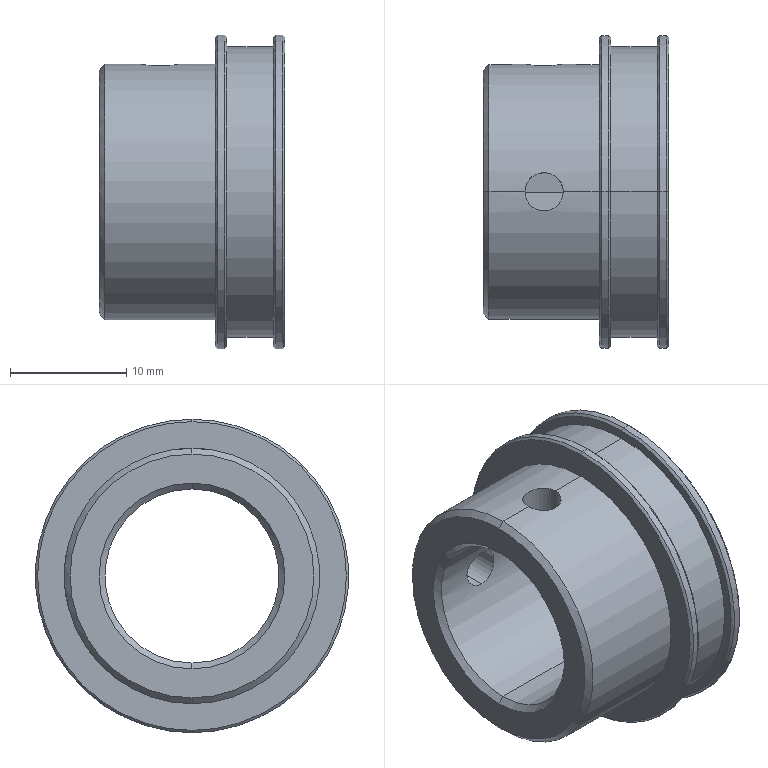Part | SolidWorks | features ICE 3, Chamfer 2, HoleWzd 2, Extrusion 1 | 1 solid | 33 faces | box 16 x 27 x 27 mm | volume 3995 mm3 | cylinder 14 | cone 14 | plane 5 | commonest cylinder face diameters 3.3 x4 27 x4 15 x2 22 x2 25 x2
STEP:
#1=CARTESIAN_POINT('',(-4.1,0.,11.));
#2=VERTEX_POINT('',#1);
#3=CARTESIAN_POINT('',(-7.4,0.,11.));
#4=VERTEX_POINT('',#3);
#5=CARTESIAN_POINT('',(-4.1,0.,11.));
#6=CARTESIAN_POINT('',(-4.1,-0.2155,11.));
#7=CARTESIAN_POINT('',(-4.143,-0.4328,10.993));
#8=CARTESIAN_POINT('',(-4.308,-0.83,10.97));
#9=CARTESIAN_POINT('',(-4.431,-1.014,10.954));
#10=CARTESIAN_POINT('',(-4.659,-1.242,10.93));
#11=CARTESIAN_POINT('',(-4.743,-1.312,10.922));
#12=CARTESIAN_POINT('',(-4.922,-1.431,10.907));
#13=CARTESIAN_POINT('',(-5.017,-1.482,10.9));
#14=CARTESIAN_POINT('',(-5.217,-1.565,10.888));
#15=CARTESIAN_POINT('',(-5.321,-1.597,10.883));
#16=CARTESIAN_POINT('',(-5.532,-1.639,10.877));
#17=CARTESIAN_POINT('',(-5.64,-1.65,10.876));
#18=CARTESIAN_POINT('',(-5.858,-1.65,10.876));
#19=CARTESIAN_POINT('',(-5.965,-1.639,10.877));
#20=CARTESIAN_POINT('',(-6.176,-1.598,10.883));
#21=CARTESIAN_POINT('',(-6.281,-1.566,10.888));
#22=CARTESIAN_POINT('',(-6.481,-1.483,10.9));
#23=CARTESIAN_POINT('',(-6.576,-1.433,10.906));
#24=CARTESIAN_POINT('',(-6.755,-1.313,10.922));
#25=CARTESIAN_POINT('',(-6.84,-1.243,10.93));
#26=CARTESIAN_POINT('',(-7.068,-1.016,10.954));
#27=CARTESIAN_POINT('',(-7.191,-0.832,10.97));
#28=CARTESIAN_POINT('',(-7.356,-0.4352,10.993));
#29=CARTESIAN_POINT('',(-7.4,-0.2183,11.));
#30=CARTESIAN_POINT('',(-7.4,0.,11.));
#31=B_SPLINE_CURVE_WITH_KNOTS('',3,(#5,#6,#7,#8,#9,#10,#11,#12,#13,#14,#15,#16,#17,#18,#19,#20,#21,#22,#23,#24,#25,#26,#27,#28,#29,#30),.UNSPECIFIED.,.F.,.F.,(4,2,2,2,2,2,2,2,2,2,2,2,4),(0.005166,0.005812,0.006457,0.00678,0.007103,0.007425,0.007748,0.008071,0.008394,0.008717,0.009039,0.009685,0.01033),.UNSPECIFIED.);
#32=EDGE_CURVE('',#2,#4,#31,.T.);
#33=ORIENTED_EDGE('',*,*,#32,.F.);
#34=CARTESIAN_POINT('',(-4.1,0.,7.5));
#35=VERTEX_POINT('',#34);
#36=CARTESIAN_POINT('',(-4.1,0.,0.));
#37=DIRECTION('',(0.,0.,-1.));
#38=VECTOR('',#37,1000.);
#39=LINE('',#36,#38);
#40=EDGE_CURVE('',#2,#35,#39,.T.);
#41=ORIENTED_EDGE('',*,*,#40,.T.);
#42=CARTESIAN_POINT('',(-7.4,0.,7.5));
#43=VERTEX_POINT('',#42);
#44=CARTESIAN_POINT('',(-4.1,0.,7.5));
#45=CARTESIAN_POINT('',(-4.1,-0.1094,7.5));
#46=CARTESIAN_POINT('',(-4.111,-0.2169,7.498));
#47=CARTESIAN_POINT('',(-4.153,-0.4282,7.489));
#48=CARTESIAN_POINT('',(-4.185,-0.5332,7.482));
#49=CARTESIAN_POINT('',(-4.268,-0.7329,7.465));
#50=CARTESIAN_POINT('',(-4.318,-0.8275,7.455));
#51=CARTESIAN_POINT('',(-4.438,-1.007,7.433));
#52=CARTESIAN_POINT('',(-4.508,-1.091,7.421));
#53=CARTESIAN_POINT('',(-4.735,-1.319,7.385));
#54=CARTESIAN_POINT('',(-4.919,-1.442,7.361));
#55=CARTESIAN_POINT('',(-5.316,-1.606,7.326));
#56=CARTESIAN_POINT('',(-5.533,-1.65,7.316));
#57=CARTESIAN_POINT('',(-5.857,-1.65,7.316));
#58=CARTESIAN_POINT('',(-5.967,-1.639,7.319));
#59=CARTESIAN_POINT('',(-6.179,-1.597,7.328));
#60=CARTESIAN_POINT('',(-6.282,-1.566,7.335));
#61=CARTESIAN_POINT('',(-6.582,-1.441,7.361));
#62=CARTESIAN_POINT('',(-6.764,-1.32,7.385));
#63=CARTESIAN_POINT('',(-6.993,-1.09,7.421));
#64=CARTESIAN_POINT('',(-7.061,-1.007,7.433));
#65=CARTESIAN_POINT('',(-7.181,-0.8286,7.455));
#66=CARTESIAN_POINT('',(-7.233,-0.7319,7.465));
#67=CARTESIAN_POINT('',(-7.315,-0.5325,7.482));
#68=CARTESIAN_POINT('',(-7.347,-0.4297,7.488));
#69=CARTESIAN_POINT('',(-7.389,-0.2174,7.498));
#70=CARTESIAN_POINT('',(-7.4,-0.1079,7.5));
#71=CARTESIAN_POINT('',(-7.4,0.,7.5));
#72=B_SPLINE_CURVE_WITH_KNOTS('',3,(#44,#45,#46,#47,#48,#49,#50,#51,#52,#53,#54,#55,#56,#57,#58,#59,#60,#61,#62,#63,#64,#65,#66,#67,#68,#69,#70,#71),.UNSPECIFIED.,.F.,.F.,(4,2,2,2,2,2,2,2,2,2,2,2,2,4),(0.,0.0003234,0.0006468,0.0009702,0.001294,0.00194,0.002587,0.002911,0.003234,0.003881,0.004204,0.004528,0.004851,0.005175),.UNSPECIFIED.);
#73=EDGE_CURVE('',#35,#43,#72,.T.);
#74=ORIENTED_EDGE('',*,*,#73,.T.);
#75=CARTESIAN_POINT('',(-7.4,0.,0.));
#76=DIRECTION('',(0.,0.,-1.));
#77=VECTOR('',#76,1000.);
#78=LINE('',#75,#77);
#79=EDGE_CURVE('',#4,#43,#78,.T.);
#80=ORIENTED_EDGE('',*,*,#79,.F.);
#81=EDGE_LOOP('',(#33,#41,#74,#80));
#82=FACE_OUTER_BOUND('',#81,.T.);
#83=CARTESIAN_POINT('',(-5.75,0.,0.));
#84=DIRECTION('',(0.,0.,-1.));
#85=DIRECTION('',(-1.,0.,0.));
#86=AXIS2_PLACEMENT_3D('',#83,#84,#85);
#87=CYLINDRICAL_SURFACE('',#86,1.65);
#88=ADVANCED_FACE('',(#82),#87,.F.);
#89=CARTESIAN_POINT('',(-5.75,10.876,1.65));
#90=VERTEX_POINT('',#89);
#91=CARTESIAN_POINT('',(-5.75,10.876,-1.65));
#92=VERTEX_POINT('',#91);
#93=CARTESIAN_POINT('',(-5.75,10.876,1.65));
#94=CARTESIAN_POINT('',(-5.965,10.876,1.65));
#95=CARTESIAN_POINT('',(-6.183,10.882,1.607));
#96=CARTESIAN_POINT('',(-6.58,10.905,1.442));
#97=CARTESIAN_POINT('',(-6.764,10.922,1.319));
#98=CARTESIAN_POINT('',(-6.992,10.946,1.092));
#99=CARTESIAN_POINT('',(-7.062,10.954,1.007));
#100=CARTESIAN_POINT('',(-7.181,10.969,0.8278));
#101=CARTESIAN_POINT('',(-7.232,10.976,0.7332));
#102=CARTESIAN_POINT('',(-7.315,10.988,0.5333));
#103=CARTESIAN_POINT('',(-7.347,10.992,0.4286));
#104=CARTESIAN_POINT('',(-7.389,10.998,0.2177));
#105=CARTESIAN_POINT('',(-7.4,11.,0.1101));
#106=CARTESIAN_POINT('',(-7.4,11.,-0.108));
#107=CARTESIAN_POINT('',(-7.389,10.998,-0.2152));
#108=CARTESIAN_POINT('',(-7.348,10.992,-0.4264));
#109=CARTESIAN_POINT('',(-7.316,10.988,-0.5314));
#110=CARTESIAN_POINT('',(-7.233,10.976,-0.731));
#111=CARTESIAN_POINT('',(-7.183,10.969,-0.8258));
#112=CARTESIAN_POINT('',(-7.063,10.954,-1.005));
#113=CARTESIAN_POINT('',(-6.993,10.946,-1.09));
#114=CARTESIAN_POINT('',(-6.766,10.922,-1.318));
#115=CARTESIAN_POINT('',(-6.582,10.906,-1.441));
#116=CARTESIAN_POINT('',(-6.185,10.882,-1.606));
#117=CARTESIAN_POINT('',(-5.968,10.876,-1.65));
#118=CARTESIAN_POINT('',(-5.75,10.876,-1.65));
#119=B_SPLINE_CURVE_WITH_KNOTS('',3,(#93,#94,#95,#96,#97,#98,#99,#100,#101,#102,#103,#104,#105,#106,#107,#108,#109,#110,#111,#112,#113,#114,#115,#116,#117,#118),.UNSPECIFIED.,.F.,.F.,(4,2,2,2,2,2,2,2,2,2,2,2,4),(0.005166,0.005812,0.006457,0.00678,0.007103,0.007425,0.007748,0.008071,0.008394,0.008717,0.009039,0.009685,0.01033),.UNSPECIFIED.);
#120=EDGE_CURVE('',#90,#92,#119,.T.);
#121=ORIENTED_EDGE('',*,*,#120,.F.);
#122=CARTESIAN_POINT('',(-5.75,7.316,1.65));
#123=VERTEX_POINT('',#122);
#124=CARTESIAN_POINT('',(-5.75,0.,1.65));
#125=DIRECTION('',(0.,-1.,0.));
#126=VECTOR('',#125,1000.);
#127=LINE('',#124,#126);
#128=EDGE_CURVE('',#90,#123,#127,.T.);
#129=ORIENTED_EDGE('',*,*,#128,.T.);
#130=CARTESIAN_POINT('',(-5.75,7.316,-1.65));
#131=VERTEX_POINT('',#130);
#132=CARTESIAN_POINT('',(-5.75,7.316,1.65));
#133=CARTESIAN_POINT('',(-5.966,7.316,1.65));
#134=CARTESIAN_POINT('',(-6.183,7.326,1.607));
#135=CARTESIAN_POINT('',(-6.481,7.352,1.483));
#136=CARTESIAN_POINT('',(-6.578,7.362,1.431));
#137=CARTESIAN_POINT('',(-6.757,7.385,1.311));
#138=CARTESIAN_POINT('',(-6.84,7.397,1.243));
#139=CARTESIAN_POINT('',(-6.992,7.421,1.091));
#140=CARTESIAN_POINT('',(-7.062,7.433,1.007));
#141=CARTESIAN_POINT('',(-7.181,7.455,0.8283));
#142=CARTESIAN_POINT('',(-7.232,7.465,0.7337));
#143=CARTESIAN_POINT('',(-7.357,7.49,0.4332));
#144=CARTESIAN_POINT('',(-7.4,7.5,0.2185));
#145=CARTESIAN_POINT('',(-7.4,7.5,-0.1082));
#146=CARTESIAN_POINT('',(-7.389,7.498,-0.2155));
#147=CARTESIAN_POINT('',(-7.347,7.489,-0.4271));
#148=CARTESIAN_POINT('',(-7.315,7.482,-0.5324));
#149=CARTESIAN_POINT('',(-7.192,7.456,-0.8312));
#150=CARTESIAN_POINT('',(-7.069,7.433,-1.014));
#151=CARTESIAN_POINT('',(-6.766,7.385,-1.318));
#152=CARTESIAN_POINT('',(-6.583,7.361,-1.441));
#153=CARTESIAN_POINT('',(-6.285,7.335,-1.565));
#154=CARTESIAN_POINT('',(-6.18,7.328,-1.597));
#155=CARTESIAN_POINT('',(-5.967,7.319,-1.639));
#156=CARTESIAN_POINT('',(-5.859,7.316,-1.65));
#157=CARTESIAN_POINT('',(-5.75,7.316,-1.65));
#158=B_SPLINE_CURVE_WITH_KNOTS('',3,(#132,#133,#134,#135,#136,#137,#138,#139,#140,#141,#142,#143,#144,#145,#146,#147,#148,#149,#150,#151,#152,#153,#154,#155,#156,#157),.UNSPECIFIED.,.F.,.F.,(4,2,2,2,2,2,2,2,2,2,2,2,4),(0.005174,0.005821,0.006144,0.006468,0.006791,0.007114,0.007761,0.008084,0.008408,0.009054,0.009701,0.01002,0.01035),.UNSPECIFIED.);
#159=EDGE_CURVE('',#123,#131,#158,.T.);
#160=ORIENTED_EDGE('',*,*,#159,.T.);
#161=CARTESIAN_POINT('',(-5.75,0.,-1.65));
#162=DIRECTION('',(0.,-1.,0.));
#163=VECTOR('',#162,1000.);
#164=LINE('',#161,#163);
#165=EDGE_CURVE('',#92,#131,#164,.T.);
#166=ORIENTED_EDGE('',*,*,#165,.F.);
#167=EDGE_LOOP('',(#121,#129,#160,#166));
#168=FACE_OUTER_BOUND('',#167,.T.);
#169=CARTESIAN_POINT('',(-5.75,0.,0.));
#170=DIRECTION('',(0.,-1.,0.));
#171=DIRECTION('',(0.,0.,-1.));
#172=AXIS2_PLACEMENT_3D('',#169,#170,#171);
#173=CYLINDRICAL_SURFACE('',#172,1.65);
#174=ADVANCED_FACE('',(#168),#173,.F.);
#175=CARTESIAN_POINT('',(4.,0.,13.3));
#176=VERTEX_POINT('',#175);
#177=CARTESIAN_POINT('',(4.,0.,-13.3));
#178=VERTEX_POINT('',#177);
#179=CARTESIAN_POINT('',(4.,0.,0.));
#180=DIRECTION('',(-1.,0.,0.));
#181=DIRECTION('',(0.,0.,-1.));
#182=AXIS2_PLACEMENT_3D('',#179,#180,#181);
#183=CIRCLE('',#182,13.3);
#184=EDGE_CURVE('',#176,#178,#183,.T.);
#185=ORIENTED_EDGE('',*,*,#184,.F.);
#186=CARTESIAN_POINT('',(4.2,0.,13.5));
#187=VERTEX_POINT('',#186);
#188=CARTESIAN_POINT('',(4.2,0.,13.5));
#189=DIRECTION('',(0.7071,0.,0.7071));
#190=VECTOR('',#189,1000.);
#191=LINE('',#188,#190);
#192=EDGE_CURVE('',#176,#187,#191,.T.);
#193=ORIENTED_EDGE('',*,*,#192,.T.);
#194=CARTESIAN_POINT('',(4.2,0.,-13.5));
#195=VERTEX_POINT('',#194);
#196=CARTESIAN_POINT('',(4.2,0.,0.));
#197=DIRECTION('',(1.,0.,0.));
#198=DIRECTION('',(0.,0.,-1.));
#199=AXIS2_PLACEMENT_3D('',#196,#197,#198);
#200=CIRCLE('',#199,13.5);
#201=EDGE_CURVE('',#195,#187,#200,.T.);
#202=ORIENTED_EDGE('',*,*,#201,.F.);
#203=CARTESIAN_POINT('',(4.2,0.,-13.5));
#204=DIRECTION('',(0.7071,0.,-0.7071));
#205=VECTOR('',#204,1000.);
#206=LINE('',#203,#205);
#207=EDGE_CURVE('',#178,#195,#206,.T.);
#208=ORIENTED_EDGE('',*,*,#207,.F.);
#209=EDGE_LOOP('',(#185,#193,#202,#208));
#210=FACE_OUTER_BOUND('',#209,.T.);
#211=CARTESIAN_POINT('',(4.2,0.,0.));
#212=DIRECTION('',(1.,0.,0.));
#213=DIRECTION('',(0.,0.,-1.));
#214=AXIS2_PLACEMENT_3D('',#211,#212,#213);
#215=CONICAL_SURFACE('',#214,13.5,0.7854);
#216=ADVANCED_FACE('',(#210),#215,.T.);
#217=CARTESIAN_POINT('',(5.,0.,-13.3));
#218=VERTEX_POINT('',#217);
#219=CARTESIAN_POINT('',(5.,0.,13.3));
#220=VERTEX_POINT('',#219);
#221=CARTESIAN_POINT('',(5.,0.,0.));
#222=DIRECTION('',(1.,0.,0.));
#223=DIRECTION('',(0.,0.,-1.));
#224=AXIS2_PLACEMENT_3D('',#221,#222,#223);
#225=CIRCLE('',#224,13.3);
#226=EDGE_CURVE('',#218,#220,#225,.T.);
#227=ORIENTED_EDGE('',*,*,#226,.F.);
#228=CARTESIAN_POINT('',(4.8,0.,-13.5));
#229=VERTEX_POINT('',#228);
#230=CARTESIAN_POINT('',(5.,0.,-13.3));
#231=DIRECTION('',(-0.7071,0.,-0.7071));
#232=VECTOR('',#231,1000.);
#233=LINE('',#230,#232);
#234=EDGE_CURVE('',#218,#229,#233,.T.);
#235=ORIENTED_EDGE('',*,*,#234,.T.);
#236=CARTESIAN_POINT('',(4.8,0.,13.5));
#237=VERTEX_POINT('',#236);
#238=CARTESIAN_POINT('',(4.8,0.,0.));
#239=DIRECTION('',(-1.,0.,0.));
#240=DIRECTION('',(0.,0.,-1.));
#241=AXIS2_PLACEMENT_3D('',#238,#239,#240);
#242=CIRCLE('',#241,13.5);
#243=EDGE_CURVE('',#237,#229,#242,.T.);
#244=ORIENTED_EDGE('',*,*,#243,.F.);
#245=CARTESIAN_POINT('',(5.,0.,13.3));
#246=DIRECTION('',(-0.7071,0.,0.7071));
#247=VECTOR('',#246,1000.);
#248=LINE('',#245,#247);
#249=EDGE_CURVE('',#220,#237,#248,.T.);
#250=ORIENTED_EDGE('',*,*,#249,.F.);
#251=EDGE_LOOP('',(#227,#235,#244,#250));
#252=FACE_OUTER_BOUND('',#251,.T.);
#253=CARTESIAN_POINT('',(5.,0.,0.));
#254=DIRECTION('',(-1.,0.,0.));
#255=DIRECTION('',(0.,0.,1.));
#256=AXIS2_PLACEMENT_3D('',#253,#254,#255);
#257=CONICAL_SURFACE('',#256,13.3,0.7854);
#258=ADVANCED_FACE('',(#252),#257,.T.);
#259=CARTESIAN_POINT('',(0.,0.,-13.3));
#260=VERTEX_POINT('',#259);
#261=CARTESIAN_POINT('',(0.,0.,13.3));
#262=VERTEX_POINT('',#261);
#263=CARTESIAN_POINT('',(0.,0.,0.));
#264=DIRECTION('',(1.,0.,0.));
#265=DIRECTION('',(0.,0.,1.));
#266=AXIS2_PLACEMENT_3D('',#263,#264,#265);
#267=CIRCLE('',#266,13.3);
#268=EDGE_CURVE('',#260,#262,#267,.T.);
#269=ORIENTED_EDGE('',*,*,#268,.F.);
#270=CARTESIAN_POINT('',(-0.2,0.,-13.5));
#271=VERTEX_POINT('',#270);
#272=CARTESIAN_POINT('',(-0.2,0.,-13.5));
#273=DIRECTION('',(-0.7071,0.,-0.7071));
#274=VECTOR('',#273,1000.);
#275=LINE('',#272,#274);
#276=EDGE_CURVE('',#260,#271,#275,.T.);
#277=ORIENTED_EDGE('',*,*,#276,.T.);
#278=CARTESIAN_POINT('',(-0.2,0.,13.5));
#279=VERTEX_POINT('',#278);
#280=CARTESIAN_POINT('',(-0.2,0.,0.));
#281=DIRECTION('',(-1.,0.,0.));
#282=DIRECTION('',(0.,0.,1.));
#283=AXIS2_PLACEMENT_3D('',#280,#281,#282);
#284=CIRCLE('',#283,13.5);
#285=EDGE_CURVE('',#279,#271,#284,.T.);
#286=ORIENTED_EDGE('',*,*,#285,.F.);
#287=CARTESIAN_POINT('',(-0.2,0.,13.5));
#288=DIRECTION('',(-0.7071,0.,0.7071));
#289=VECTOR('',#288,1000.);
#290=LINE('',#287,#289);
#291=EDGE_CURVE('',#262,#279,#290,.T.);
#292=ORIENTED_EDGE('',*,*,#291,.F.);
#293=EDGE_LOOP('',(#269,#277,#286,#292));
#294=FACE_OUTER_BOUND('',#293,.T.);
#295=CARTESIAN_POINT('',(-0.2,0.,0.));
#296=DIRECTION('',(-1.,0.,0.));
#297=DIRECTION('',(0.,0.,1.));
#298=AXIS2_PLACEMENT_3D('',#295,#296,#297);
#299=CONICAL_SURFACE('',#298,13.5,0.7854);
#300=ADVANCED_FACE('',(#294),#299,.T.);
#301=CARTESIAN_POINT('',(-1.,0.,13.3));
#302=VERTEX_POINT('',#301);
#303=CARTESIAN_POINT('',(-1.,0.,-13.3));
#304=VERTEX_POINT('',#303);
#305=CARTESIAN_POINT('',(-1.,0.,0.));
#306=DIRECTION('',(-1.,0.,0.));
#307=DIRECTION('',(0.,0.,1.));
#308=AXIS2_PLACEMENT_3D('',#305,#306,#307);
#309=CIRCLE('',#308,13.3);
#310=EDGE_CURVE('',#302,#304,#309,.T.);
#311=ORIENTED_EDGE('',*,*,#310,.F.);
#312=CARTESIAN_POINT('',(-0.8,0.,13.5));
#313=VERTEX_POINT('',#312);
#314=CARTESIAN_POINT('',(-1.,0.,13.3));
#315=DIRECTION('',(0.7071,0.,0.7071));
#316=VECTOR('',#315,1000.);
#317=LINE('',#314,#316);
#318=EDGE_CURVE('',#302,#313,#317,.T.);
#319=ORIENTED_EDGE('',*,*,#318,.T.);
#320=CARTESIAN_POINT('',(-0.8,0.,-13.5));
#321=VERTEX_POINT('',#320);
#322=CARTESIAN_POINT('',(-0.8,0.,0.));
#323=DIRECTION('',(1.,0.,0.));
#324=DIRECTION('',(0.,0.,1.));
#325=AXIS2_PLACEMENT_3D('',#322,#323,#324);
#326=CIRCLE('',#325,13.5);
#327=EDGE_CURVE('',#321,#313,#326,.T.);
#328=ORIENTED_EDGE('',*,*,#327,.F.);
#329=CARTESIAN_POINT('',(-1.,0.,-13.3));
#330=DIRECTION('',(0.7071,0.,-0.7071));
#331=VECTOR('',#330,1000.);
#332=LINE('',#329,#331);
#333=EDGE_CURVE('',#304,#321,#332,.T.);
#334=ORIENTED_EDGE('',*,*,#333,.F.);
#335=EDGE_LOOP('',(#311,#319,#328,#334));
#336=FACE_OUTER_BOUND('',#335,.T.);
#337=CARTESIAN_POINT('',(-1.,0.,0.));
#338=DIRECTION('',(1.,0.,0.));
#339=DIRECTION('',(0.,0.,-1.));
#340=AXIS2_PLACEMENT_3D('',#337,#338,#339);
#341=CONICAL_SURFACE('',#340,13.3,0.7854);
#342=ADVANCED_FACE('',(#336),#341,.T.);
#343=CARTESIAN_POINT('',(4.5,0.,7.5));
#344=VERTEX_POINT('',#343);
#345=CARTESIAN_POINT('',(4.5,0.,-7.5));
#346=VERTEX_POINT('',#345);
#347=CARTESIAN_POINT('',(4.5,0.,0.));
#348=DIRECTION('',(1.,0.,0.));
#349=DIRECTION('',(0.,0.,-1.));
#350=AXIS2_PLACEMENT_3D('',#347,#348,#349);
#351=CIRCLE('',#350,7.5);
#352=EDGE_CURVE('',#344,#346,#351,.T.);
#353=ORIENTED_EDGE('',*,*,#352,.F.);
#354=CARTESIAN_POINT('',(5.,0.,8.));
#355=VERTEX_POINT('',#354);
#356=CARTESIAN_POINT('',(4.5,0.,7.5));
#357=DIRECTION('',(0.7071,0.,0.7071));
#358=VECTOR('',#357,1000.);
#359=LINE('',#356,#358);
#360=EDGE_CURVE('',#344,#355,#359,.T.);
#361=ORIENTED_EDGE('',*,*,#360,.T.);
#362=CARTESIAN_POINT('',(5.,0.,-8.));
#363=VERTEX_POINT('',#362);
#364=CARTESIAN_POINT('',(5.,0.,0.));
#365=DIRECTION('',(-1.,0.,0.));
#366=DIRECTION('',(0.,0.,-1.));
#367=AXIS2_PLACEMENT_3D('',#364,#365,#366);
#368=CIRCLE('',#367,8.);
#369=EDGE_CURVE('',#363,#355,#368,.T.);
#370=ORIENTED_EDGE('',*,*,#369,.F.);
#371=CARTESIAN_POINT('',(4.5,0.,-7.5));
#372=DIRECTION('',(0.7071,0.,-0.7071));
#373=VECTOR('',#372,1000.);
#374=LINE('',#371,#373);
#375=EDGE_CURVE('',#346,#363,#374,.T.);
#376=ORIENTED_EDGE('',*,*,#375,.F.);
#377=EDGE_LOOP('',(#353,#361,#370,#376));
#378=FACE_OUTER_BOUND('',#377,.T.);
#379=CARTESIAN_POINT('',(4.5,0.,0.));
#380=DIRECTION('',(1.,0.,0.));
#381=DIRECTION('',(0.,0.,-1.));
#382=AXIS2_PLACEMENT_3D('',#379,#380,#381);
#383=CONICAL_SURFACE('',#382,7.5,0.7854);
#384=ADVANCED_FACE('',(#378),#383,.F.);
#385=CARTESIAN_POINT('',(-11.,0.,10.5));
#386=VERTEX_POINT('',#385);
#387=CARTESIAN_POINT('',(-11.,0.,-10.5));
#388=VERTEX_POINT('',#387);
#389=CARTESIAN_POINT('',(-11.,0.,0.));
#390=DIRECTION('',(-1.,0.,0.));
#391=DIRECTION('',(0.,0.,1.));
#392=AXIS2_PLACEMENT_3D('',#389,#390,#391);
#393=CIRCLE('',#392,10.5);
#394=EDGE_CURVE('',#386,#388,#393,.T.);
#395=ORIENTED_EDGE('',*,*,#394,.F.);
#396=CARTESIAN_POINT('',(-10.5,0.,11.));
#397=VERTEX_POINT('',#396);
#398=CARTESIAN_POINT('',(-11.,0.,10.5));
#399=DIRECTION('',(0.7071,0.,0.7071));
#400=VECTOR('',#399,1000.);
#401=LINE('',#398,#400);
#402=EDGE_CURVE('',#386,#397,#401,.T.);
#403=ORIENTED_EDGE('',*,*,#402,.T.);
#404=CARTESIAN_POINT('',(-10.5,0.,-11.));
#405=VERTEX_POINT('',#404);
#406=CARTESIAN_POINT('',(-10.5,0.,0.));
#407=DIRECTION('',(1.,0.,0.));
#408=DIRECTION('',(0.,0.,1.));
#409=AXIS2_PLACEMENT_3D('',#406,#407,#408);
#410=CIRCLE('',#409,11.);
#411=EDGE_CURVE('',#405,#397,#410,.T.);
#412=ORIENTED_EDGE('',*,*,#411,.F.);
#413=CARTESIAN_POINT('',(-11.,0.,-10.5));
#414=DIRECTION('',(0.7071,0.,-0.7071));
#415=VECTOR('',#414,1000.);
#416=LINE('',#413,#415);
#417=EDGE_CURVE('',#388,#405,#416,.T.);
#418=ORIENTED_EDGE('',*,*,#417,.F.);
#419=EDGE_LOOP('',(#395,#403,#412,#418));
#420=FACE_OUTER_BOUND('',#419,.T.);
#421=CARTESIAN_POINT('',(-11.,0.,0.));
#422=DIRECTION('',(1.,0.,0.));
#423=DIRECTION('',(0.,0.,-1.));
#424=AXIS2_PLACEMENT_3D('',#421,#422,#423);
#425=CONICAL_SURFACE('',#424,10.5,0.7854);
#426=ADVANCED_FACE('',(#420),#425,.T.);
#427=CARTESIAN_POINT('',(-10.5,0.,-7.5));
#428=VERTEX_POINT('',#427);
#429=CARTESIAN_POINT('',(-10.5,0.,7.5));
#430=VERTEX_POINT('',#429);
#431=CARTESIAN_POINT('',(-10.5,0.,0.));
#432=DIRECTION('',(-1.,0.,0.));
#433=DIRECTION('',(0.,0.,1.));
#434=AXIS2_PLACEMENT_3D('',#431,#432,#433);
#435=CIRCLE('',#434,7.5);
#436=EDGE_CURVE('',#428,#430,#435,.T.);
#437=ORIENTED_EDGE('',*,*,#436,.F.);
#438=CARTESIAN_POINT('',(-11.,0.,-8.));
#439=VERTEX_POINT('',#438);
#440=CARTESIAN_POINT('',(-10.5,0.,-7.5));
#441=DIRECTION('',(-0.7071,0.,-0.7071));
#442=VECTOR('',#441,1000.);
#443=LINE('',#440,#442);
#444=EDGE_CURVE('',#428,#439,#443,.T.);
#445=ORIENTED_EDGE('',*,*,#444,.T.);
#446=CARTESIAN_POINT('',(-11.,0.,8.));
#447=VERTEX_POINT('',#446);
#448=CARTESIAN_POINT('',(-11.,0.,0.));
#449=DIRECTION('',(1.,0.,0.));
#450=DIRECTION('',(0.,0.,1.));
#451=AXIS2_PLACEMENT_3D('',#448,#449,#450);
#452=CIRCLE('',#451,8.);
#453=EDGE_CURVE('',#447,#439,#452,.T.);
#454=ORIENTED_EDGE('',*,*,#453,.F.);
#455=CARTESIAN_POINT('',(-10.5,0.,7.5));
#456=DIRECTION('',(-0.7071,0.,0.7071));
#457=VECTOR('',#456,1000.);
#458=LINE('',#455,#457);
#459=EDGE_CURVE('',#430,#447,#458,.T.);
#460=ORIENTED_EDGE('',*,*,#459,.F.);
#461=EDGE_LOOP('',(#437,#445,#454,#460));
#462=FACE_OUTER_BOUND('',#461,.T.);
#463=CARTESIAN_POINT('',(-10.5,0.,0.));
#464=DIRECTION('',(-1.,0.,0.));
#465=DIRECTION('',(0.,0.,1.));
#466=AXIS2_PLACEMENT_3D('',#463,#464,#465);
#467=CONICAL_SURFACE('',#466,7.5,0.7854);
#468=ADVANCED_FACE('',(#462),#467,.F.);
#469=CARTESIAN_POINT('',(-5.75,10.876,-1.65));
#470=CARTESIAN_POINT('',(-5.641,10.876,-1.65));
#471=CARTESIAN_POINT('',(-5.533,10.877,-1.639));
#472=CARTESIAN_POINT('',(-5.322,10.883,-1.597));
#473=CARTESIAN_POINT('',(-5.217,10.888,-1.565));
#474=CARTESIAN_POINT('',(-5.018,10.9,-1.483));
#475=CARTESIAN_POINT('',(-4.923,10.907,-1.432));
#476=CARTESIAN_POINT('',(-4.744,10.922,-1.312));
#477=CARTESIAN_POINT('',(-4.659,10.93,-1.242));
#478=CARTESIAN_POINT('',(-4.431,10.954,-1.014));
#479=CARTESIAN_POINT('',(-4.308,10.97,-0.8306));
#480=CARTESIAN_POINT('',(-4.144,10.993,-0.4336));
#481=CARTESIAN_POINT('',(-4.1,11.,-0.2162));
#482=CARTESIAN_POINT('',(-4.1,11.,0.1072));
#483=CARTESIAN_POINT('',(-4.111,10.998,0.2167));
#484=CARTESIAN_POINT('',(-4.153,10.992,0.4284));
#485=CARTESIAN_POINT('',(-4.184,10.988,0.5314));
#486=CARTESIAN_POINT('',(-4.267,10.976,0.7313));
#487=CARTESIAN_POINT('',(-4.319,10.969,0.8277));
#488=CARTESIAN_POINT('',(-4.438,10.954,1.006));
#489=CARTESIAN_POINT('',(-4.506,10.946,1.09));
#490=CARTESIAN_POINT('',(-4.66,10.93,1.244));
#491=CARTESIAN_POINT('',(-4.743,10.922,1.312));
#492=CARTESIAN_POINT('',(-4.922,10.907,1.431));
#493=CARTESIAN_POINT('',(-5.018,10.9,1.483));
#494=CARTESIAN_POINT('',(-5.218,10.888,1.566));
#495=CARTESIAN_POINT('',(-5.321,10.883,1.597));
#496=CARTESIAN_POINT('',(-5.533,10.877,1.639));
#497=CARTESIAN_POINT('',(-5.642,10.876,1.65));
#498=CARTESIAN_POINT('',(-5.75,10.876,1.65));
#499=B_SPLINE_CURVE_WITH_KNOTS('',3,(#469,#470,#471,#472,#473,#474,#475,#476,#477,#478,#479,#480,#481,#482,#483,#484,#485,#486,#487,#488,#489,#490,#491,#492,#493,#494,#495,#496,#497,#498),.UNSPECIFIED.,.F.,.F.,(4,2,2,2,2,2,2,2,2,2,2,2,2,2,4),(0.,0.0003229,0.0006457,0.0009686,0.001291,0.001937,0.002583,0.002906,0.003229,0.003552,0.003874,0.004197,0.00452,0.004843,0.005166),.UNSPECIFIED.);
#500=EDGE_CURVE('',#92,#90,#499,.T.);
#501=ORIENTED_EDGE('',*,*,#500,.T.);
#502=ORIENTED_EDGE('',*,*,#120,.T.);
#503=EDGE_LOOP('',(#501,#502));
#504=FACE_BOUND('',#503,.T.);
#505=ORIENTED_EDGE('',*,*,#411,.T.);
#506=CARTESIAN_POINT('',(-11.,0.,11.));
#507=DIRECTION('',(1.,0.,0.));
#508=VECTOR('',#507,1000.);
#509=LINE('',#506,#508);
#510=EDGE_CURVE('',#397,#4,#509,.T.);
#511=ORIENTED_EDGE('',*,*,#510,.T.);
#512=CARTESIAN_POINT('',(-7.4,0.,11.));
#513=CARTESIAN_POINT('',(-7.4,0.1092,11.));
#514=CARTESIAN_POINT('',(-7.389,0.2165,10.998));
#515=CARTESIAN_POINT('',(-7.347,0.4276,10.992));
#516=CARTESIAN_POINT('',(-7.315,0.5325,10.988));
#517=CARTESIAN_POINT('',(-7.233,0.7323,10.976));
#518=CARTESIAN_POINT('',(-7.182,0.827,10.969));
#519=CARTESIAN_POINT('',(-7.062,1.006,10.954));
#520=CARTESIAN_POINT('',(-6.992,1.091,10.946));
#521=CARTESIAN_POINT('',(-6.764,1.319,10.922));
#522=CARTESIAN_POINT('',(-6.581,1.442,10.905));
#523=CARTESIAN_POINT('',(-6.184,1.606,10.882));
#524=CARTESIAN_POINT('',(-5.966,1.65,10.876));
#525=CARTESIAN_POINT('',(-5.643,1.65,10.876));
#526=CARTESIAN_POINT('',(-5.533,1.639,10.877));
#527=CARTESIAN_POINT('',(-5.322,1.597,10.883));
#528=CARTESIAN_POINT('',(-5.219,1.566,10.888));
#529=CARTESIAN_POINT('',(-5.019,1.483,10.9));
#530=CARTESIAN_POINT('',(-4.922,1.431,10.907));
#531=CARTESIAN_POINT('',(-4.744,1.312,10.922));
#532=CARTESIAN_POINT('',(-4.66,1.244,10.93));
#533=CARTESIAN_POINT('',(-4.506,1.09,10.946));
#534=CARTESIAN_POINT('',(-4.438,1.007,10.954));
#535=CARTESIAN_POINT('',(-4.319,0.8281,10.969));
#536=CARTESIAN_POINT('',(-4.267,0.7316,10.976));
#537=CARTESIAN_POINT('',(-4.184,0.5319,10.988));
#538=CARTESIAN_POINT('',(-4.153,0.429,10.992));
#539=CARTESIAN_POINT('',(-4.111,0.2172,10.998));
#540=CARTESIAN_POINT('',(-4.1,0.1078,11.));
#541=CARTESIAN_POINT('',(-4.1,0.,11.));
#542=B_SPLINE_CURVE_WITH_KNOTS('',3,(#512,#513,#514,#515,#516,#517,#518,#519,#520,#521,#522,#523,#524,#525,#526,#527,#528,#529,#530,#531,#532,#533,#534,#535,#536,#537,#538,#539,#540,#541),.UNSPECIFIED.,.F.,.F.,(4,2,2,2,2,2,2,2,2,2,2,2,2,2,4),(0.,0.0003229,0.0006457,0.0009686,0.001291,0.001937,0.002583,0.002906,0.003229,0.003552,0.003874,0.004197,0.00452,0.004843,0.005166),.UNSPECIFIED.);
#543=EDGE_CURVE('',#4,#2,#542,.T.);
#544=ORIENTED_EDGE('',*,*,#543,.T.);
#545=CARTESIAN_POINT('',(-1.,0.,11.));
#546=VERTEX_POINT('',#545);
#547=CARTESIAN_POINT('',(-11.,0.,11.));
#548=DIRECTION('',(1.,0.,0.));
#549=VECTOR('',#548,1000.);
#550=LINE('',#547,#549);
#551=EDGE_CURVE('',#2,#546,#550,.T.);
#552=ORIENTED_EDGE('',*,*,#551,.T.);
#553=CARTESIAN_POINT('',(-1.,0.,-11.));
#554=VERTEX_POINT('',#553);
#555=CARTESIAN_POINT('',(-1.,0.,0.));
#556=DIRECTION('',(-1.,0.,0.));
#557=DIRECTION('',(0.,0.,1.));
#558=AXIS2_PLACEMENT_3D('',#555,#556,#557);
#559=CIRCLE('',#558,11.);
#560=EDGE_CURVE('',#546,#554,#559,.T.);
#561=ORIENTED_EDGE('',*,*,#560,.T.);
#562=CARTESIAN_POINT('',(-11.,0.,-11.));
#563=DIRECTION('',(1.,0.,0.));
#564=VECTOR('',#563,1000.);
#565=LINE('',#562,#564);
#566=EDGE_CURVE('',#405,#554,#565,.T.);
#567=ORIENTED_EDGE('',*,*,#566,.F.);
#568=EDGE_LOOP('',(#505,#511,#544,#552,#561,#567));
#569=FACE_OUTER_BOUND('',#568,.T.);
#570=CARTESIAN_POINT('',(-11.,0.,0.));
#571=DIRECTION('',(1.,0.,0.));
#572=DIRECTION('',(0.,0.,-1.));
#573=AXIS2_PLACEMENT_3D('',#570,#571,#572);
#574=CYLINDRICAL_SURFACE('',#573,11.);
#575=ADVANCED_FACE('',(#504,#569),#574,.T.);
#576=ORIENTED_EDGE('',*,*,#327,.T.);
#577=CARTESIAN_POINT('',(-1.,0.,13.5));
#578=DIRECTION('',(1.,0.,0.));
#579=VECTOR('',#578,1000.);
#580=LINE('',#577,#579);
#581=EDGE_CURVE('',#313,#279,#580,.T.);
#582=ORIENTED_EDGE('',*,*,#581,.T.);
#583=ORIENTED_EDGE('',*,*,#285,.T.);
#584=CARTESIAN_POINT('',(-1.,0.,-13.5));
#585=DIRECTION('',(1.,0.,0.));
#586=VECTOR('',#585,1000.);
#587=LINE('',#584,#586);
#588=EDGE_CURVE('',#321,#271,#587,.T.);
#589=ORIENTED_EDGE('',*,*,#588,.F.);
#590=EDGE_LOOP('',(#576,#582,#583,#589));
#591=FACE_OUTER_BOUND('',#590,.T.);
#592=CARTESIAN_POINT('',(-1.,0.,0.));
#593=DIRECTION('',(1.,0.,0.));
#594=DIRECTION('',(0.,0.,-1.));
#595=AXIS2_PLACEMENT_3D('',#592,#593,#594);
#596=CYLINDRICAL_SURFACE('',#595,13.5);
#597=ADVANCED_FACE('',(#591),#596,.T.);
#598=ORIENTED_EDGE('',*,*,#243,.T.);
#599=CARTESIAN_POINT('',(5.,0.,-13.5));
#600=DIRECTION('',(-1.,0.,0.));
#601=VECTOR('',#600,1000.);
#602=LINE('',#599,#601);
#603=EDGE_CURVE('',#229,#195,#602,.T.);
#604=ORIENTED_EDGE('',*,*,#603,.T.);
#605=ORIENTED_EDGE('',*,*,#201,.T.);
#606=CARTESIAN_POINT('',(5.,0.,13.5));
#607=DIRECTION('',(-1.,0.,0.));
#608=VECTOR('',#607,1000.);
#609=LINE('',#606,#608);
#610=EDGE_CURVE('',#237,#187,#609,.T.);
#611=ORIENTED_EDGE('',*,*,#610,.F.);
#612=EDGE_LOOP('',(#598,#604,#605,#611));
#613=FACE_OUTER_BOUND('',#612,.T.);
#614=CARTESIAN_POINT('',(5.,0.,0.));
#615=DIRECTION('',(-1.,0.,0.));
#616=DIRECTION('',(0.,0.,1.));
#617=AXIS2_PLACEMENT_3D('',#614,#615,#616);
#618=CYLINDRICAL_SURFACE('',#617,13.5);
#619=ADVANCED_FACE('',(#613),#618,.T.);
#620=ORIENTED_EDGE('',*,*,#352,.T.);
#621=CARTESIAN_POINT('',(4.,0.,-7.5));
#622=DIRECTION('',(-1.,0.,0.));
#623=VECTOR('',#622,1000.);
#624=LINE('',#621,#623);
#625=EDGE_CURVE('',#346,#428,#624,.T.);
#626=ORIENTED_EDGE('',*,*,#625,.T.);
#627=ORIENTED_EDGE('',*,*,#436,.T.);
#628=CARTESIAN_POINT('',(4.,0.,7.5));
#629=DIRECTION('',(-1.,0.,0.));
#630=VECTOR('',#629,1000.);
#631=LINE('',#628,#630);
#632=EDGE_CURVE('',#43,#430,#631,.T.);
#633=ORIENTED_EDGE('',*,*,#632,.F.);
#634=ORIENTED_EDGE('',*,*,#73,.F.);
#635=CARTESIAN_POINT('',(4.,0.,7.5));
#636=DIRECTION('',(-1.,0.,0.));
#637=VECTOR('',#636,1000.);
#638=LINE('',#635,#637);
#639=EDGE_CURVE('',#344,#35,#638,.T.);
#640=ORIENTED_EDGE('',*,*,#639,.F.);
#641=EDGE_LOOP('',(#620,#626,#627,#633,#634,#640));
#642=FACE_OUTER_BOUND('',#641,.T.);
#643=CARTESIAN_POINT('',(4.,0.,0.));
#644=DIRECTION('',(-1.,0.,0.));
#645=DIRECTION('',(0.,0.,1.));
#646=AXIS2_PLACEMENT_3D('',#643,#644,#645);
#647=CYLINDRICAL_SURFACE('',#646,7.5);
#648=ADVANCED_FACE('',(#642),#647,.F.);
#649=CARTESIAN_POINT('',(4.,0.,-12.5));
#650=VERTEX_POINT('',#649);
#651=CARTESIAN_POINT('',(4.,0.,12.5));
#652=VERTEX_POINT('',#651);
#653=CARTESIAN_POINT('',(4.,0.,0.));
#654=DIRECTION('',(1.,0.,0.));
#655=DIRECTION('',(0.,0.,-1.));
#656=AXIS2_PLACEMENT_3D('',#653,#654,#655);
#657=CIRCLE('',#656,12.5);
#658=EDGE_CURVE('',#650,#652,#657,.T.);
#659=ORIENTED_EDGE('',*,*,#658,.F.);
#660=CARTESIAN_POINT('',(0.,0.,-12.5));
#661=VERTEX_POINT('',#660);
#662=CARTESIAN_POINT('',(4.,0.,-12.5));
#663=DIRECTION('',(-1.,0.,0.));
#664=VECTOR('',#663,1000.);
#665=LINE('',#662,#664);
#666=EDGE_CURVE('',#650,#661,#665,.T.);
#667=ORIENTED_EDGE('',*,*,#666,.T.);
#668=CARTESIAN_POINT('',(0.,0.,12.5));
#669=VERTEX_POINT('',#668);
#670=CARTESIAN_POINT('',(0.,0.,0.));
#671=DIRECTION('',(-1.,0.,0.));
#672=DIRECTION('',(0.,0.,1.));
#673=AXIS2_PLACEMENT_3D('',#670,#671,#672);
#674=CIRCLE('',#673,12.5);
#675=EDGE_CURVE('',#669,#661,#674,.T.);
#676=ORIENTED_EDGE('',*,*,#675,.F.);
#677=CARTESIAN_POINT('',(4.,0.,12.5));
#678=DIRECTION('',(-1.,0.,0.));
#679=VECTOR('',#678,1000.);
#680=LINE('',#677,#679);
#681=EDGE_CURVE('',#652,#669,#680,.T.);
#682=ORIENTED_EDGE('',*,*,#681,.F.);
#683=EDGE_LOOP('',(#659,#667,#676,#682));
#684=FACE_OUTER_BOUND('',#683,.T.);
#685=CARTESIAN_POINT('',(4.,0.,0.));
#686=DIRECTION('',(-1.,0.,0.));
#687=DIRECTION('',(0.,0.,1.));
#688=AXIS2_PLACEMENT_3D('',#685,#686,#687);
#689=CYLINDRICAL_SURFACE('',#688,12.5);
#690=ADVANCED_FACE('',(#684),#689,.T.);
#691=CARTESIAN_POINT('',(-1.,0.,0.));
#692=DIRECTION('',(-1.,0.,0.));
#693=DIRECTION('',(0.,0.,1.));
#694=AXIS2_PLACEMENT_3D('',#691,#692,#693);
#695=CIRCLE('',#694,13.3);
#696=EDGE_CURVE('',#304,#302,#695,.T.);
#697=ORIENTED_EDGE('',*,*,#696,.T.);
#698=ORIENTED_EDGE('',*,*,#310,.T.);
#699=EDGE_LOOP('',(#697,#698));
#700=FACE_OUTER_BOUND('',#699,.T.);
#701=CARTESIAN_POINT('',(-1.,0.,0.));
#702=DIRECTION('',(-1.,0.,0.));
#703=DIRECTION('',(0.,0.,1.));
#704=AXIS2_PLACEMENT_3D('',#701,#702,#703);
#705=CIRCLE('',#704,11.);
#706=EDGE_CURVE('',#554,#546,#705,.T.);
#707=ORIENTED_EDGE('',*,*,#706,.F.);
#708=ORIENTED_EDGE('',*,*,#560,.F.);
#709=EDGE_LOOP('',(#707,#708));
#710=FACE_BOUND('',#709,.T.);
#711=CARTESIAN_POINT('',(-1.,0.,0.));
#712=DIRECTION('',(-1.,0.,0.));
#713=DIRECTION('',(0.,0.,1.));
#714=AXIS2_PLACEMENT_3D('',#711,#712,#713);
#715=PLANE('',#714);
#716=ADVANCED_FACE('',(#700,#710),#715,.T.);
#717=ORIENTED_EDGE('',*,*,#666,.F.);
#718=CARTESIAN_POINT('',(4.,0.,0.));
#719=DIRECTION('',(1.,0.,0.));
#720=DIRECTION('',(0.,0.,-1.));
#721=AXIS2_PLACEMENT_3D('',#718,#719,#720);
#722=CIRCLE('',#721,12.5);
#723=EDGE_CURVE('',#652,#650,#722,.T.);
#724=ORIENTED_EDGE('',*,*,#723,.F.);
#725=ORIENTED_EDGE('',*,*,#681,.T.);
#726=CARTESIAN_POINT('',(0.,0.,0.));
#727=DIRECTION('',(-1.,0.,0.));
#728=DIRECTION('',(0.,0.,1.));
#729=AXIS2_PLACEMENT_3D('',#726,#727,#728);
#730=CIRCLE('',#729,12.5);
#731=EDGE_CURVE('',#661,#669,#730,.T.);
#732=ORIENTED_EDGE('',*,*,#731,.F.);
#733=EDGE_LOOP('',(#717,#724,#725,#732));
#734=FACE_OUTER_BOUND('',#733,.T.);
#735=CARTESIAN_POINT('',(4.,0.,0.));
#736=DIRECTION('',(-1.,0.,0.));
#737=DIRECTION('',(0.,0.,1.));
#738=AXIS2_PLACEMENT_3D('',#735,#736,#737);
#739=CYLINDRICAL_SURFACE('',#738,12.5);
#740=ADVANCED_FACE('',(#734),#739,.T.);
#741=ORIENTED_EDGE('',*,*,#625,.F.);
#742=CARTESIAN_POINT('',(4.5,0.,0.));
#743=DIRECTION('',(1.,0.,0.));
#744=DIRECTION('',(0.,0.,-1.));
#745=AXIS2_PLACEMENT_3D('',#742,#743,#744);
#746=CIRCLE('',#745,7.5);
#747=EDGE_CURVE('',#346,#344,#746,.T.);
#748=ORIENTED_EDGE('',*,*,#747,.T.);
#749=ORIENTED_EDGE('',*,*,#639,.T.);
#750=CARTESIAN_POINT('',(-7.4,0.,7.5));
#751=CARTESIAN_POINT('',(-7.4,0.2157,7.5));
#752=CARTESIAN_POINT('',(-7.357,0.4334,7.49));
#753=CARTESIAN_POINT('',(-7.233,0.7314,7.465));
#754=CARTESIAN_POINT('',(-7.181,0.8278,7.455));
#755=CARTESIAN_POINT('',(-7.061,1.007,7.433));
#756=CARTESIAN_POINT('',(-6.993,1.09,7.421));
#757=CARTESIAN_POINT('',(-6.841,1.242,7.397));
#758=CARTESIAN_POINT('',(-6.757,1.312,7.385));
#759=CARTESIAN_POINT('',(-6.578,1.431,7.362));
#760=CARTESIAN_POINT('',(-6.484,1.482,7.352));
#761=CARTESIAN_POINT('',(-6.183,1.607,7.326));
#762=CARTESIAN_POINT('',(-5.968,1.65,7.316));
#763=CARTESIAN_POINT('',(-5.642,1.65,7.316));
#764=CARTESIAN_POINT('',(-5.534,1.639,7.319));
#765=CARTESIAN_POINT('',(-5.323,1.597,7.328));
#766=CARTESIAN_POINT('',(-5.218,1.565,7.335));
#767=CARTESIAN_POINT('',(-4.919,1.442,7.361));
#768=CARTESIAN_POINT('',(-4.736,1.319,7.385));
#769=CARTESIAN_POINT('',(-4.432,1.016,7.432));
#770=CARTESIAN_POINT('',(-4.309,0.8326,7.456));
#771=CARTESIAN_POINT('',(-4.185,0.5349,7.482));
#772=CARTESIAN_POINT('',(-4.153,0.43,7.488));
#773=CARTESIAN_POINT('',(-4.111,0.2172,7.498));
#774=CARTESIAN_POINT('',(-4.1,0.1094,7.5));
#775=CARTESIAN_POINT('',(-4.1,0.,7.5));
#776=B_SPLINE_CURVE_WITH_KNOTS('',3,(#750,#751,#752,#753,#754,#755,#756,#757,#758,#759,#760,#761,#762,#763,#764,#765,#766,#767,#768,#769,#770,#771,#772,#773,#774,#775),.UNSPECIFIED.,.F.,.F.,(4,2,2,2,2,2,2,2,2,2,2,2,4),(0.005175,0.005821,0.006144,0.006468,0.006791,0.007114,0.007761,0.008084,0.008408,0.009054,0.009701,0.01002,0.01035),.UNSPECIFIED.);
#777=EDGE_CURVE('',#43,#35,#776,.T.);
#778=ORIENTED_EDGE('',*,*,#777,.F.);
#779=ORIENTED_EDGE('',*,*,#632,.T.);
#780=CARTESIAN_POINT('',(-10.5,0.,0.));
#781=DIRECTION('',(-1.,0.,0.));
#782=DIRECTION('',(0.,0.,1.));
#783=AXIS2_PLACEMENT_3D('',#780,#781,#782);
#784=CIRCLE('',#783,7.5);
#785=EDGE_CURVE('',#430,#428,#784,.T.);
#786=ORIENTED_EDGE('',*,*,#785,.T.);
#787=EDGE_LOOP('',(#741,#748,#749,#778,#779,#786));
#788=FACE_OUTER_BOUND('',#787,.T.);
#789=CARTESIAN_POINT('',(-5.75,7.316,-1.65));
#790=CARTESIAN_POINT('',(-5.641,7.316,-1.65));
#791=CARTESIAN_POINT('',(-5.533,7.319,-1.639));
#792=CARTESIAN_POINT('',(-5.322,7.328,-1.597));
#793=CARTESIAN_POINT('',(-5.217,7.335,-1.565));
#794=CARTESIAN_POINT('',(-5.017,7.352,-1.482));
#795=CARTESIAN_POINT('',(-4.922,7.362,-1.432));
#796=CARTESIAN_POINT('',(-4.743,7.385,-1.312));
#797=CARTESIAN_POINT('',(-4.659,7.397,-1.242));
#798=CARTESIAN_POINT('',(-4.431,7.433,-1.015));
#799=CARTESIAN_POINT('',(-4.309,7.456,-0.8311));
#800=CARTESIAN_POINT('',(-4.144,7.49,-0.4343));
#801=CARTESIAN_POINT('',(-4.1,7.5,-0.2166));
#802=CARTESIAN_POINT('',(-4.1,7.5,0.1073));
#803=CARTESIAN_POINT('',(-4.111,7.498,0.2171));
#804=CARTESIAN_POINT('',(-4.153,7.488,0.429));
#805=CARTESIAN_POINT('',(-4.184,7.482,0.532));
#806=CARTESIAN_POINT('',(-4.309,7.456,0.8323));
#807=CARTESIAN_POINT('',(-4.43,7.433,1.014));
#808=CARTESIAN_POINT('',(-4.66,7.397,1.244));
#809=CARTESIAN_POINT('',(-4.743,7.385,1.312));
#810=CARTESIAN_POINT('',(-4.921,7.362,1.431));
#811=CARTESIAN_POINT('',(-5.018,7.352,1.483));
#812=CARTESIAN_POINT('',(-5.217,7.335,1.565));
#813=CARTESIAN_POINT('',(-5.32,7.328,1.597));
#814=CARTESIAN_POINT('',(-5.533,7.319,1.639));
#815=CARTESIAN_POINT('',(-5.642,7.316,1.65));
#816=CARTESIAN_POINT('',(-5.75,7.316,1.65));
#817=B_SPLINE_CURVE_WITH_KNOTS('',3,(#789,#790,#791,#792,#793,#794,#795,#796,#797,#798,#799,#800,#801,#802,#803,#804,#805,#806,#807,#808,#809,#810,#811,#812,#813,#814,#815,#816),.UNSPECIFIED.,.F.,.F.,(4,2,2,2,2,2,2,2,2,2,2,2,2,4),(0.,0.0003234,0.0006468,0.0009702,0.001294,0.00194,0.002587,0.002911,0.003234,0.003881,0.004204,0.004528,0.004851,0.005174),.UNSPECIFIED.);
#818=EDGE_CURVE('',#131,#123,#817,.T.);
#819=ORIENTED_EDGE('',*,*,#818,.F.);
#820=ORIENTED_EDGE('',*,*,#159,.F.);
#821=EDGE_LOOP('',(#819,#820));
#822=FACE_BOUND('',#821,.T.);
#823=CARTESIAN_POINT('',(4.,0.,0.));
#824=DIRECTION('',(-1.,0.,0.));
#825=DIRECTION('',(0.,0.,1.));
#826=AXIS2_PLACEMENT_3D('',#823,#824,#825);
#827=CYLINDRICAL_SURFACE('',#826,7.5);
#828=ADVANCED_FACE('',(#788,#822),#827,.F.);
#829=CARTESIAN_POINT('',(4.,0.,0.));
#830=DIRECTION('',(-1.,0.,0.));
#831=DIRECTION('',(0.,0.,-1.));
#832=AXIS2_PLACEMENT_3D('',#829,#830,#831);
#833=CIRCLE('',#832,13.3);
#834=EDGE_CURVE('',#178,#176,#833,.T.);
#835=ORIENTED_EDGE('',*,*,#834,.T.);
#836=ORIENTED_EDGE('',*,*,#184,.T.);
#837=EDGE_LOOP('',(#835,#836));
#838=FACE_OUTER_BOUND('',#837,.T.);
#839=ORIENTED_EDGE('',*,*,#723,.T.);
#840=ORIENTED_EDGE('',*,*,#658,.T.);
#841=EDGE_LOOP('',(#839,#840));
#842=FACE_BOUND('',#841,.T.);
#843=CARTESIAN_POINT('',(4.,0.,0.));
#844=DIRECTION('',(1.,0.,0.));
#845=DIRECTION('',(0.,0.,-1.));
#846=AXIS2_PLACEMENT_3D('',#843,#844,#845);
#847=PLANE('',#846);
#848=ADVANCED_FACE('',(#838,#842),#847,.F.);
#849=CARTESIAN_POINT('',(5.,0.,0.));
#850=DIRECTION('',(1.,0.,0.));
#851=DIRECTION('',(0.,0.,-1.));
#852=AXIS2_PLACEMENT_3D('',#849,#850,#851);
#853=CIRCLE('',#852,13.3);
#854=EDGE_CURVE('',#220,#218,#853,.T.);
#855=ORIENTED_EDGE('',*,*,#854,.T.);
#856=ORIENTED_EDGE('',*,*,#226,.T.);
#857=EDGE_LOOP('',(#855,#856));
#858=FACE_OUTER_BOUND('',#857,.T.);
#859=ORIENTED_EDGE('',*,*,#369,.T.);
#860=CARTESIAN_POINT('',(5.,0.,0.));
#861=DIRECTION('',(-1.,0.,0.));
#862=DIRECTION('',(0.,0.,-1.));
#863=AXIS2_PLACEMENT_3D('',#860,#861,#862);
#864=CIRCLE('',#863,8.);
#865=EDGE_CURVE('',#355,#363,#864,.T.);
#866=ORIENTED_EDGE('',*,*,#865,.T.);
#867=EDGE_LOOP('',(#859,#866));
#868=FACE_BOUND('',#867,.T.);
#869=CARTESIAN_POINT('',(5.,0.,0.));
#870=DIRECTION('',(1.,0.,0.));
#871=DIRECTION('',(0.,0.,-1.));
#872=AXIS2_PLACEMENT_3D('',#869,#870,#871);
#873=PLANE('',#872);
#874=ADVANCED_FACE('',(#858,#868),#873,.T.);
#875=ORIENTED_EDGE('',*,*,#603,.F.);
#876=CARTESIAN_POINT('',(4.8,0.,0.));
#877=DIRECTION('',(-1.,0.,0.));
#878=DIRECTION('',(0.,0.,-1.));
#879=AXIS2_PLACEMENT_3D('',#876,#877,#878);
#880=CIRCLE('',#879,13.5);
#881=EDGE_CURVE('',#229,#237,#880,.T.);
#882=ORIENTED_EDGE('',*,*,#881,.T.);
#883=ORIENTED_EDGE('',*,*,#610,.T.);
#884=CARTESIAN_POINT('',(4.2,0.,0.));
#885=DIRECTION('',(1.,0.,0.));
#886=DIRECTION('',(0.,0.,-1.));
#887=AXIS2_PLACEMENT_3D('',#884,#885,#886);
#888=CIRCLE('',#887,13.5);
#889=EDGE_CURVE('',#187,#195,#888,.T.);
#890=ORIENTED_EDGE('',*,*,#889,.T.);
#891=EDGE_LOOP('',(#875,#882,#883,#890));
#892=FACE_OUTER_BOUND('',#891,.T.);
#893=CARTESIAN_POINT('',(5.,0.,0.));
#894=DIRECTION('',(-1.,0.,0.));
#895=DIRECTION('',(0.,0.,1.));
#896=AXIS2_PLACEMENT_3D('',#893,#894,#895);
#897=CYLINDRICAL_SURFACE('',#896,13.5);
#898=ADVANCED_FACE('',(#892),#897,.T.);
#899=CARTESIAN_POINT('',(0.,0.,0.));
#900=DIRECTION('',(1.,0.,0.));
#901=DIRECTION('',(0.,0.,1.));
#902=AXIS2_PLACEMENT_3D('',#899,#900,#901);
#903=CIRCLE('',#902,13.3);
#904=EDGE_CURVE('',#262,#260,#903,.T.);
#905=ORIENTED_EDGE('',*,*,#904,.T.);
#906=ORIENTED_EDGE('',*,*,#268,.T.);
#907=EDGE_LOOP('',(#905,#906));
#908=FACE_OUTER_BOUND('',#907,.T.);
#909=ORIENTED_EDGE('',*,*,#675,.T.);
#910=ORIENTED_EDGE('',*,*,#731,.T.);
#911=EDGE_LOOP('',(#909,#910));
#912=FACE_BOUND('',#911,.T.);
#913=CARTESIAN_POINT('',(0.,0.,0.));
#914=DIRECTION('',(-1.,0.,0.));
#915=DIRECTION('',(0.,0.,1.));
#916=AXIS2_PLACEMENT_3D('',#913,#914,#915);
#917=PLANE('',#916);
#918=ADVANCED_FACE('',(#908,#912),#917,.F.);
#919=ORIENTED_EDGE('',*,*,#581,.F.);
#920=CARTESIAN_POINT('',(-0.8,0.,0.));
#921=DIRECTION('',(1.,0.,0.));
#922=DIRECTION('',(0.,0.,1.));
#923=AXIS2_PLACEMENT_3D('',#920,#921,#922);
#924=CIRCLE('',#923,13.5);
#925=EDGE_CURVE('',#313,#321,#924,.T.);
#926=ORIENTED_EDGE('',*,*,#925,.T.);
#927=ORIENTED_EDGE('',*,*,#588,.T.);
#928=CARTESIAN_POINT('',(-0.2,0.,0.));
#929=DIRECTION('',(-1.,0.,0.));
#930=DIRECTION('',(0.,0.,1.));
#931=AXIS2_PLACEMENT_3D('',#928,#929,#930);
#932=CIRCLE('',#931,13.5);
#933=EDGE_CURVE('',#271,#279,#932,.T.);
#934=ORIENTED_EDGE('',*,*,#933,.T.);
#935=EDGE_LOOP('',(#919,#926,#927,#934));
#936=FACE_OUTER_BOUND('',#935,.T.);
#937=CARTESIAN_POINT('',(-1.,0.,0.));
#938=DIRECTION('',(1.,0.,0.));
#939=DIRECTION('',(0.,0.,-1.));
#940=AXIS2_PLACEMENT_3D('',#937,#938,#939);
#941=CYLINDRICAL_SURFACE('',#940,13.5);
#942=ADVANCED_FACE('',(#936),#941,.T.);
#943=ORIENTED_EDGE('',*,*,#453,.T.);
#944=CARTESIAN_POINT('',(-11.,0.,0.));
#945=DIRECTION('',(1.,0.,0.));
#946=DIRECTION('',(0.,0.,1.));
#947=AXIS2_PLACEMENT_3D('',#944,#945,#946);
#948=CIRCLE('',#947,8.);
#949=EDGE_CURVE('',#439,#447,#948,.T.);
#950=ORIENTED_EDGE('',*,*,#949,.T.);
#951=EDGE_LOOP('',(#943,#950));
#952=FACE_BOUND('',#951,.T.);
#953=CARTESIAN_POINT('',(-11.,0.,0.));
#954=DIRECTION('',(-1.,0.,0.));
#955=DIRECTION('',(0.,0.,1.));
#956=AXIS2_PLACEMENT_3D('',#953,#954,#955);
#957=CIRCLE('',#956,10.5);
#958=EDGE_CURVE('',#388,#386,#957,.T.);
#959=ORIENTED_EDGE('',*,*,#958,.T.);
#960=ORIENTED_EDGE('',*,*,#394,.T.);
#961=EDGE_LOOP('',(#959,#960));
#962=FACE_OUTER_BOUND('',#961,.T.);
#963=CARTESIAN_POINT('',(-11.,0.,0.));
#964=DIRECTION('',(-1.,0.,0.));
#965=DIRECTION('',(0.,0.,1.));
#966=AXIS2_PLACEMENT_3D('',#963,#964,#965);
#967=PLANE('',#966);
#968=ADVANCED_FACE('',(#952,#962),#967,.T.);
#969=ORIENTED_EDGE('',*,*,#510,.F.);
#970=CARTESIAN_POINT('',(-10.5,0.,0.));
#971=DIRECTION('',(1.,0.,0.));
#972=DIRECTION('',(0.,0.,1.));
#973=AXIS2_PLACEMENT_3D('',#970,#971,#972);
#974=CIRCLE('',#973,11.);
#975=EDGE_CURVE('',#397,#405,#974,.T.);
#976=ORIENTED_EDGE('',*,*,#975,.T.);
#977=ORIENTED_EDGE('',*,*,#566,.T.);
#978=ORIENTED_EDGE('',*,*,#706,.T.);
#979=ORIENTED_EDGE('',*,*,#551,.F.);
#980=ORIENTED_EDGE('',*,*,#32,.T.);
#981=EDGE_LOOP('',(#969,#976,#977,#978,#979,#980));
#982=FACE_OUTER_BOUND('',#981,.T.);
#983=CARTESIAN_POINT('',(-11.,0.,0.));
#984=DIRECTION('',(1.,0.,0.));
#985=DIRECTION('',(0.,0.,-1.));
#986=AXIS2_PLACEMENT_3D('',#983,#984,#985);
#987=CYLINDRICAL_SURFACE('',#986,11.);
#988=ADVANCED_FACE('',(#982),#987,.T.);
#989=ORIENTED_EDGE('',*,*,#444,.F.);
#990=ORIENTED_EDGE('',*,*,#785,.F.);
#991=ORIENTED_EDGE('',*,*,#459,.T.);
#992=ORIENTED_EDGE('',*,*,#949,.F.);
#993=EDGE_LOOP('',(#989,#990,#991,#992));
#994=FACE_OUTER_BOUND('',#993,.T.);
#995=CARTESIAN_POINT('',(-10.5,0.,0.));
#996=DIRECTION('',(-1.,0.,0.));
#997=DIRECTION('',(0.,0.,1.));
#998=AXIS2_PLACEMENT_3D('',#995,#996,#997);
#999=CONICAL_SURFACE('',#998,7.5,0.7854);
#1000=ADVANCED_FACE('',(#994),#999,.F.);
#1001=ORIENTED_EDGE('',*,*,#402,.F.);
#1002=ORIENTED_EDGE('',*,*,#958,.F.);
#1003=ORIENTED_EDGE('',*,*,#417,.T.);
#1004=ORIENTED_EDGE('',*,*,#975,.F.);
#1005=EDGE_LOOP('',(#1001,#1002,#1003,#1004));
#1006=FACE_OUTER_BOUND('',#1005,.T.);
#1007=CARTESIAN_POINT('',(-11.,0.,0.));
#1008=DIRECTION('',(1.,0.,0.));
#1009=DIRECTION('',(0.,0.,-1.));
#1010=AXIS2_PLACEMENT_3D('',#1007,#1008,#1009);
#1011=CONICAL_SURFACE('',#1010,10.5,0.7854);
#1012=ADVANCED_FACE('',(#1006),#1011,.T.);
#1013=ORIENTED_EDGE('',*,*,#360,.F.);
#1014=ORIENTED_EDGE('',*,*,#747,.F.);
#1015=ORIENTED_EDGE('',*,*,#375,.T.);
#1016=ORIENTED_EDGE('',*,*,#865,.F.);
#1017=EDGE_LOOP('',(#1013,#1014,#1015,#1016));
#1018=FACE_OUTER_BOUND('',#1017,.T.);
#1019=CARTESIAN_POINT('',(4.5,0.,0.));
#1020=DIRECTION('',(1.,0.,0.));
#1021=DIRECTION('',(0.,0.,-1.));
#1022=AXIS2_PLACEMENT_3D('',#1019,#1020,#1021);
#1023=CONICAL_SURFACE('',#1022,7.5,0.7854);
#1024=ADVANCED_FACE('',(#1018),#1023,.F.);
#1025=ORIENTED_EDGE('',*,*,#318,.F.);
#1026=ORIENTED_EDGE('',*,*,#696,.F.);
#1027=ORIENTED_EDGE('',*,*,#333,.T.);
#1028=ORIENTED_EDGE('',*,*,#925,.F.);
#1029=EDGE_LOOP('',(#1025,#1026,#1027,#1028));
#1030=FACE_OUTER_BOUND('',#1029,.T.);
#1031=CARTESIAN_POINT('',(-1.,0.,0.));
#1032=DIRECTION('',(1.,0.,0.));
#1033=DIRECTION('',(0.,0.,-1.));
#1034=AXIS2_PLACEMENT_3D('',#1031,#1032,#1033);
#1035=CONICAL_SURFACE('',#1034,13.3,0.7854);
#1036=ADVANCED_FACE('',(#1030),#1035,.T.);
#1037=ORIENTED_EDGE('',*,*,#276,.F.);
#1038=ORIENTED_EDGE('',*,*,#904,.F.);
#1039=ORIENTED_EDGE('',*,*,#291,.T.);
#1040=ORIENTED_EDGE('',*,*,#933,.F.);
#1041=EDGE_LOOP('',(#1037,#1038,#1039,#1040));
#1042=FACE_OUTER_BOUND('',#1041,.T.);
#1043=CARTESIAN_POINT('',(-0.2,0.,0.));
#1044=DIRECTION('',(-1.,0.,0.));
#1045=DIRECTION('',(0.,0.,1.));
#1046=AXIS2_PLACEMENT_3D('',#1043,#1044,#1045);
#1047=CONICAL_SURFACE('',#1046,13.5,0.7854);
#1048=ADVANCED_FACE('',(#1042),#1047,.T.);
#1049=ORIENTED_EDGE('',*,*,#234,.F.);
#1050=ORIENTED_EDGE('',*,*,#854,.F.);
#1051=ORIENTED_EDGE('',*,*,#249,.T.);
#1052=ORIENTED_EDGE('',*,*,#881,.F.);
#1053=EDGE_LOOP('',(#1049,#1050,#1051,#1052));
#1054=FACE_OUTER_BOUND('',#1053,.T.);
#1055=CARTESIAN_POINT('',(5.,0.,0.));
#1056=DIRECTION('',(-1.,0.,0.));
#1057=DIRECTION('',(0.,0.,1.));
#1058=AXIS2_PLACEMENT_3D('',#1055,#1056,#1057);
#1059=CONICAL_SURFACE('',#1058,13.3,0.7854);
#1060=ADVANCED_FACE('',(#1054),#1059,.T.);
#1061=ORIENTED_EDGE('',*,*,#192,.F.);
#1062=ORIENTED_EDGE('',*,*,#834,.F.);
#1063=ORIENTED_EDGE('',*,*,#207,.T.);
#1064=ORIENTED_EDGE('',*,*,#889,.F.);
#1065=EDGE_LOOP('',(#1061,#1062,#1063,#1064));
#1066=FACE_OUTER_BOUND('',#1065,.T.);
#1067=CARTESIAN_POINT('',(4.2,0.,0.));
#1068=DIRECTION('',(1.,0.,0.));
#1069=DIRECTION('',(0.,0.,-1.));
#1070=AXIS2_PLACEMENT_3D('',#1067,#1068,#1069);
#1071=CONICAL_SURFACE('',#1070,13.5,0.7854);
#1072=ADVANCED_FACE('',(#1066),#1071,.T.);
#1073=ORIENTED_EDGE('',*,*,#128,.F.);
#1074=ORIENTED_EDGE('',*,*,#500,.F.);
#1075=ORIENTED_EDGE('',*,*,#165,.T.);
#1076=ORIENTED_EDGE('',*,*,#818,.T.);
#1077=EDGE_LOOP('',(#1073,#1074,#1075,#1076));
#1078=FACE_OUTER_BOUND('',#1077,.T.);
#1079=CARTESIAN_POINT('',(-5.75,0.,0.));
#1080=DIRECTION('',(0.,-1.,0.));
#1081=DIRECTION('',(0.,0.,-1.));
#1082=AXIS2_PLACEMENT_3D('',#1079,#1080,#1081);
#1083=CYLINDRICAL_SURFACE('',#1082,1.65);
#1084=ADVANCED_FACE('',(#1078),#1083,.F.);
#1085=ORIENTED_EDGE('',*,*,#40,.F.);
#1086=ORIENTED_EDGE('',*,*,#543,.F.);
#1087=ORIENTED_EDGE('',*,*,#79,.T.);
#1088=ORIENTED_EDGE('',*,*,#777,.T.);
#1089=EDGE_LOOP('',(#1085,#1086,#1087,#1088));
#1090=FACE_OUTER_BOUND('',#1089,.T.);
#1091=CARTESIAN_POINT('',(-5.75,0.,0.));
#1092=DIRECTION('',(0.,0.,-1.));
#1093=DIRECTION('',(-1.,0.,0.));
#1094=AXIS2_PLACEMENT_3D('',#1091,#1092,#1093);
#1095=CYLINDRICAL_SURFACE('',#1094,1.65);
#1096=ADVANCED_FACE('',(#1090),#1095,.F.);
#1097=CLOSED_SHELL('',(#88,#174,#216,#258,#300,#342,#384,#426,#468,#575,#597,#619,#648,#690,#716,#740,#828,#848,#874,#898,#918,#942,#968,#988,#1000,#1012,#1024,#1036,#1048,#1060,#1072,#1084,#1096));
#1098=MANIFOLD_SOLID_BREP('',#1097);
#1099=CARTESIAN_POINT('',(0.,0.,0.));
#1100=DIRECTION('',(0.,0.,1.));
#1101=DIRECTION('',(1.,0.,0.));
#1102=AXIS2_PLACEMENT_3D('',#1099,#1100,#1101);
#1103=(LENGTH_UNIT()NAMED_UNIT(*)SI_UNIT(.MILLI.,.METRE.));
#1104=UNCERTAINTY_MEASURE_WITH_UNIT(LENGTH_MEASURE(0.00001),#1103,'','');
#1105=(NAMED_UNIT(*)PLANE_ANGLE_UNIT()SI_UNIT($,.RADIAN.));
#1106=(NAMED_UNIT(*)SI_UNIT($,.STERADIAN.)SOLID_ANGLE_UNIT());
#1107=(GEOMETRIC_REPRESENTATION_CONTEXT(3)GLOBAL_UNCERTAINTY_ASSIGNED_CONTEXT((#1104))GLOBAL_UNIT_ASSIGNED_CONTEXT((#1103,#1105,#1106))REPRESENTATION_CONTEXT('',''));
#1108=ADVANCED_BREP_SHAPE_REPRESENTATION('',(#1098,#1102),#1107);